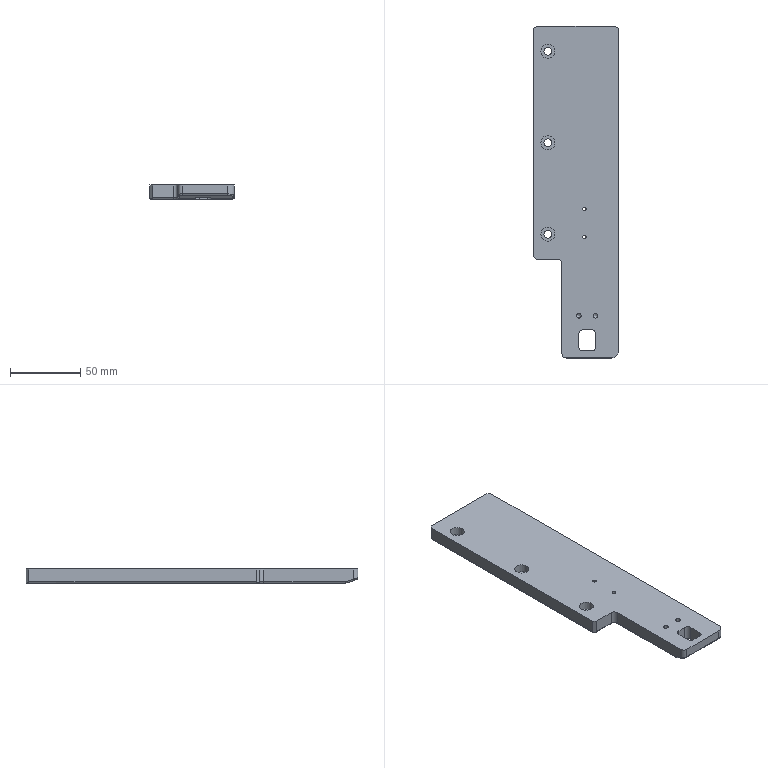Part | 1 solid | 52 faces | box 60 x 236 x 10 mm | volume 123281 mm3 | cylinder 26 | plane 19 | torus 3 | cone 2 | spline 2 | commonest cylinder face diameters 2 x7 6 x6 10 x6 5.5 x3 2.459 x2 3.242 x2